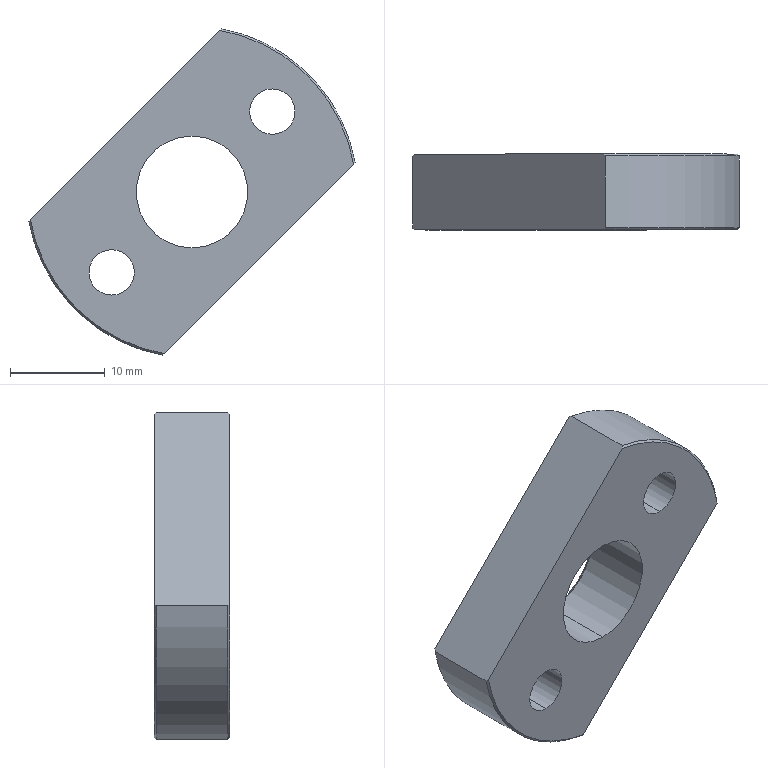Part | SolidWorks | features 3DProfileFeature 2, Chamfer 2, HoleWzd 2, ICE 2, Fillet 1, Revolution 1 | 1 solid | 24 faces | box 34.452 x 8 x 34.452 mm | volume 3811 mm3 | cylinder 12 | cone 6 | plane 6 | commonest cylinder face diameters 4.8 x4 8 x4 11.8 x2 35 x2
STEP:
#1=CARTESIAN_POINT('',(0.,23.5,-5.9));
#2=VERTEX_POINT('',#1);
#3=CARTESIAN_POINT('',(0.,23.5,5.9));
#4=VERTEX_POINT('',#3);
#5=CARTESIAN_POINT('',(0.,23.5,0.));
#6=DIRECTION('',(0.,1.,0.));
#7=DIRECTION('',(0.,0.,-1.));
#8=AXIS2_PLACEMENT_3D('',#5,#6,#7);
#9=CIRCLE('',#8,5.9);
#10=EDGE_CURVE('',#2,#4,#9,.T.);
#11=ORIENTED_EDGE('',*,*,#10,.F.);
#12=CARTESIAN_POINT('',(0.,24.,-6.4));
#13=VERTEX_POINT('',#12);
#14=CARTESIAN_POINT('',(0.,23.5,-5.9));
#15=DIRECTION('',(0.,0.7071,-0.7071));
#16=VECTOR('',#15,1000.);
#17=LINE('',#14,#16);
#18=EDGE_CURVE('',#2,#13,#17,.T.);
#19=ORIENTED_EDGE('',*,*,#18,.T.);
#20=CARTESIAN_POINT('',(0.,24.,6.4));
#21=VERTEX_POINT('',#20);
#22=CARTESIAN_POINT('',(0.,24.,0.));
#23=DIRECTION('',(0.,-1.,0.));
#24=DIRECTION('',(0.,0.,-1.));
#25=AXIS2_PLACEMENT_3D('',#22,#23,#24);
#26=CIRCLE('',#25,6.4);
#27=EDGE_CURVE('',#21,#13,#26,.T.);
#28=ORIENTED_EDGE('',*,*,#27,.F.);
#29=CARTESIAN_POINT('',(0.,23.5,5.9));
#30=DIRECTION('',(0.,0.7071,0.7071));
#31=VECTOR('',#30,1000.);
#32=LINE('',#29,#31);
#33=EDGE_CURVE('',#4,#21,#32,.T.);
#34=ORIENTED_EDGE('',*,*,#33,.F.);
#35=EDGE_LOOP('',(#11,#19,#28,#34));
#36=FACE_OUTER_BOUND('',#35,.T.);
#37=CARTESIAN_POINT('',(0.,23.5,0.));
#38=DIRECTION('',(0.,1.,0.));
#39=DIRECTION('',(0.,0.,1.));
#40=AXIS2_PLACEMENT_3D('',#37,#38,#39);
#41=CONICAL_SURFACE('',#40,5.9,0.7854);
#42=ADVANCED_FACE('',(#36),#41,.F.);
#43=CARTESIAN_POINT('',(-8.485,19.4,-12.485));
#44=VERTEX_POINT('',#43);
#45=CARTESIAN_POINT('',(-8.485,19.4,-4.485));
#46=VERTEX_POINT('',#45);
#47=CARTESIAN_POINT('',(-8.485,19.4,-8.485));
#48=DIRECTION('',(0.,1.,0.));
#49=DIRECTION('',(0.,0.,1.));
#50=AXIS2_PLACEMENT_3D('',#47,#48,#49);
#51=CIRCLE('',#50,4.);
#52=EDGE_CURVE('',#44,#46,#51,.T.);
#53=ORIENTED_EDGE('',*,*,#52,.F.);
#54=CARTESIAN_POINT('',(-8.485,24.,-12.485));
#55=VERTEX_POINT('',#54);
#56=CARTESIAN_POINT('',(-8.485,24.,-12.485));
#57=DIRECTION('',(0.,1.,0.));
#58=VECTOR('',#57,1000.);
#59=LINE('',#56,#58);
#60=EDGE_CURVE('',#44,#55,#59,.T.);
#61=ORIENTED_EDGE('',*,*,#60,.T.);
#62=CARTESIAN_POINT('',(-8.485,24.,-4.485));
#63=VERTEX_POINT('',#62);
#64=CARTESIAN_POINT('',(-8.485,24.,-8.485));
#65=DIRECTION('',(0.,1.,0.));
#66=DIRECTION('',(0.,0.,1.));
#67=AXIS2_PLACEMENT_3D('',#64,#65,#66);
#68=CIRCLE('',#67,4.);
#69=EDGE_CURVE('',#55,#63,#68,.T.);
#70=ORIENTED_EDGE('',*,*,#69,.T.);
#71=CARTESIAN_POINT('',(-8.485,24.,-4.485));
#72=DIRECTION('',(0.,1.,0.));
#73=VECTOR('',#72,1000.);
#74=LINE('',#71,#73);
#75=EDGE_CURVE('',#46,#63,#74,.T.);
#76=ORIENTED_EDGE('',*,*,#75,.F.);
#77=EDGE_LOOP('',(#53,#61,#70,#76));
#78=FACE_OUTER_BOUND('',#77,.T.);
#79=CARTESIAN_POINT('',(-8.485,24.,-8.485));
#80=DIRECTION('',(0.,1.,0.));
#81=DIRECTION('',(0.,0.,1.));
#82=AXIS2_PLACEMENT_3D('',#79,#80,#81);
#83=CYLINDRICAL_SURFACE('',#82,4.);
#84=ADVANCED_FACE('',(#78),#83,.F.);
#85=CARTESIAN_POINT('',(-8.485,16.,-10.885));
#86=VERTEX_POINT('',#85);
#87=CARTESIAN_POINT('',(-8.485,16.,-6.085));
#88=VERTEX_POINT('',#87);
#89=CARTESIAN_POINT('',(-8.485,16.,-8.485));
#90=DIRECTION('',(0.,1.,0.));
#91=DIRECTION('',(0.,0.,1.));
#92=AXIS2_PLACEMENT_3D('',#89,#90,#91);
#93=CIRCLE('',#92,2.4);
#94=EDGE_CURVE('',#86,#88,#93,.T.);
#95=ORIENTED_EDGE('',*,*,#94,.F.);
#96=CARTESIAN_POINT('',(-8.485,19.4,-10.885));
#97=VERTEX_POINT('',#96);
#98=CARTESIAN_POINT('',(-8.485,24.,-10.885));
#99=DIRECTION('',(0.,1.,0.));
#100=VECTOR('',#99,1000.);
#101=LINE('',#98,#100);
#102=EDGE_CURVE('',#86,#97,#101,.T.);
#103=ORIENTED_EDGE('',*,*,#102,.T.);
#104=CARTESIAN_POINT('',(-8.485,19.4,-6.085));
#105=VERTEX_POINT('',#104);
#106=CARTESIAN_POINT('',(-8.485,19.4,-8.485));
#107=DIRECTION('',(0.,1.,0.));
#108=DIRECTION('',(0.,0.,1.));
#109=AXIS2_PLACEMENT_3D('',#106,#107,#108);
#110=CIRCLE('',#109,2.4);
#111=EDGE_CURVE('',#97,#105,#110,.T.);
#112=ORIENTED_EDGE('',*,*,#111,.T.);
#113=CARTESIAN_POINT('',(-8.485,24.,-6.085));
#114=DIRECTION('',(0.,1.,0.));
#115=VECTOR('',#114,1000.);
#116=LINE('',#113,#115);
#117=EDGE_CURVE('',#88,#105,#116,.T.);
#118=ORIENTED_EDGE('',*,*,#117,.F.);
#119=EDGE_LOOP('',(#95,#103,#112,#118));
#120=FACE_OUTER_BOUND('',#119,.T.);
#121=CARTESIAN_POINT('',(-8.485,24.,-8.485));
#122=DIRECTION('',(0.,1.,0.));
#123=DIRECTION('',(0.,0.,1.));
#124=AXIS2_PLACEMENT_3D('',#121,#122,#123);
#125=CYLINDRICAL_SURFACE('',#124,2.4);
#126=ADVANCED_FACE('',(#120),#125,.F.);
#127=CARTESIAN_POINT('',(8.485,19.4,4.485));
#128=VERTEX_POINT('',#127);
#129=CARTESIAN_POINT('',(8.485,19.4,12.485));
#130=VERTEX_POINT('',#129);
#131=CARTESIAN_POINT('',(8.485,19.4,8.485));
#132=DIRECTION('',(0.,1.,0.));
#133=DIRECTION('',(0.,0.,1.));
#134=AXIS2_PLACEMENT_3D('',#131,#132,#133);
#135=CIRCLE('',#134,4.);
#136=EDGE_CURVE('',#128,#130,#135,.T.);
#137=ORIENTED_EDGE('',*,*,#136,.F.);
#138=CARTESIAN_POINT('',(8.485,24.,4.485));
#139=VERTEX_POINT('',#138);
#140=CARTESIAN_POINT('',(8.485,24.,4.485));
#141=DIRECTION('',(0.,1.,0.));
#142=VECTOR('',#141,1000.);
#143=LINE('',#140,#142);
#144=EDGE_CURVE('',#128,#139,#143,.T.);
#145=ORIENTED_EDGE('',*,*,#144,.T.);
#146=CARTESIAN_POINT('',(8.485,24.,12.485));
#147=VERTEX_POINT('',#146);
#148=CARTESIAN_POINT('',(8.485,24.,8.485));
#149=DIRECTION('',(0.,1.,0.));
#150=DIRECTION('',(0.,0.,1.));
#151=AXIS2_PLACEMENT_3D('',#148,#149,#150);
#152=CIRCLE('',#151,4.);
#153=EDGE_CURVE('',#139,#147,#152,.T.);
#154=ORIENTED_EDGE('',*,*,#153,.T.);
#155=CARTESIAN_POINT('',(8.485,24.,12.485));
#156=DIRECTION('',(0.,1.,0.));
#157=VECTOR('',#156,1000.);
#158=LINE('',#155,#157);
#159=EDGE_CURVE('',#130,#147,#158,.T.);
#160=ORIENTED_EDGE('',*,*,#159,.F.);
#161=EDGE_LOOP('',(#137,#145,#154,#160));
#162=FACE_OUTER_BOUND('',#161,.T.);
#163=CARTESIAN_POINT('',(8.485,24.,8.485));
#164=DIRECTION('',(0.,1.,0.));
#165=DIRECTION('',(0.,0.,1.));
#166=AXIS2_PLACEMENT_3D('',#163,#164,#165);
#167=CYLINDRICAL_SURFACE('',#166,4.);
#168=ADVANCED_FACE('',(#162),#167,.F.);
#169=CARTESIAN_POINT('',(8.485,16.,6.085));
#170=VERTEX_POINT('',#169);
#171=CARTESIAN_POINT('',(8.485,16.,10.885));
#172=VERTEX_POINT('',#171);
#173=CARTESIAN_POINT('',(8.485,16.,8.485));
#174=DIRECTION('',(0.,1.,0.));
#175=DIRECTION('',(0.,0.,1.));
#176=AXIS2_PLACEMENT_3D('',#173,#174,#175);
#177=CIRCLE('',#176,2.4);
#178=EDGE_CURVE('',#170,#172,#177,.T.);
#179=ORIENTED_EDGE('',*,*,#178,.F.);
#180=CARTESIAN_POINT('',(8.485,19.4,6.085));
#181=VERTEX_POINT('',#180);
#182=CARTESIAN_POINT('',(8.485,24.,6.085));
#183=DIRECTION('',(0.,1.,0.));
#184=VECTOR('',#183,1000.);
#185=LINE('',#182,#184);
#186=EDGE_CURVE('',#170,#181,#185,.T.);
#187=ORIENTED_EDGE('',*,*,#186,.T.);
#188=CARTESIAN_POINT('',(8.485,19.4,10.885));
#189=VERTEX_POINT('',#188);
#190=CARTESIAN_POINT('',(8.485,19.4,8.485));
#191=DIRECTION('',(0.,1.,0.));
#192=DIRECTION('',(0.,0.,1.));
#193=AXIS2_PLACEMENT_3D('',#190,#191,#192);
#194=CIRCLE('',#193,2.4);
#195=EDGE_CURVE('',#181,#189,#194,.T.);
#196=ORIENTED_EDGE('',*,*,#195,.T.);
#197=CARTESIAN_POINT('',(8.485,24.,10.885));
#198=DIRECTION('',(0.,1.,0.));
#199=VECTOR('',#198,1000.);
#200=LINE('',#197,#199);
#201=EDGE_CURVE('',#172,#189,#200,.T.);
#202=ORIENTED_EDGE('',*,*,#201,.F.);
#203=EDGE_LOOP('',(#179,#187,#196,#202));
#204=FACE_OUTER_BOUND('',#203,.T.);
#205=CARTESIAN_POINT('',(8.485,24.,8.485));
#206=DIRECTION('',(0.,1.,0.));
#207=DIRECTION('',(0.,0.,1.));
#208=AXIS2_PLACEMENT_3D('',#205,#206,#207);
#209=CYLINDRICAL_SURFACE('',#208,2.4);
#210=ADVANCED_FACE('',(#204),#209,.F.);
#211=CARTESIAN_POINT('',(0.,16.,-5.9));
#212=VERTEX_POINT('',#211);
#213=CARTESIAN_POINT('',(0.,16.,5.9));
#214=VERTEX_POINT('',#213);
#215=CARTESIAN_POINT('',(0.,16.,0.));
#216=DIRECTION('',(0.,1.,0.));
#217=DIRECTION('',(0.,0.,-1.));
#218=AXIS2_PLACEMENT_3D('',#215,#216,#217);
#219=CIRCLE('',#218,5.9);
#220=EDGE_CURVE('',#212,#214,#219,.T.);
#221=ORIENTED_EDGE('',*,*,#220,.F.);
#222=CARTESIAN_POINT('',(0.,24.,-5.9));
#223=DIRECTION('',(0.,1.,0.));
#224=VECTOR('',#223,1000.);
#225=LINE('',#222,#224);
#226=EDGE_CURVE('',#212,#2,#225,.T.);
#227=ORIENTED_EDGE('',*,*,#226,.T.);
#228=ORIENTED_EDGE('',*,*,#10,.T.);
#229=CARTESIAN_POINT('',(0.,24.,5.9));
#230=DIRECTION('',(0.,1.,0.));
#231=VECTOR('',#230,1000.);
#232=LINE('',#229,#231);
#233=EDGE_CURVE('',#214,#4,#232,.T.);
#234=ORIENTED_EDGE('',*,*,#233,.F.);
#235=EDGE_LOOP('',(#221,#227,#228,#234));
#236=FACE_OUTER_BOUND('',#235,.T.);
#237=CARTESIAN_POINT('',(0.,24.,0.));
#238=DIRECTION('',(0.,1.,0.));
#239=DIRECTION('',(0.,0.,1.));
#240=AXIS2_PLACEMENT_3D('',#237,#238,#239);
#241=CYLINDRICAL_SURFACE('',#240,5.9);
#242=ADVANCED_FACE('',(#236),#241,.F.);
#243=ORIENTED_EDGE('',*,*,#226,.F.);
#244=CARTESIAN_POINT('',(0.,16.,0.));
#245=DIRECTION('',(0.,1.,0.));
#246=DIRECTION('',(0.,0.,-1.));
#247=AXIS2_PLACEMENT_3D('',#244,#245,#246);
#248=CIRCLE('',#247,5.9);
#249=EDGE_CURVE('',#214,#212,#248,.T.);
#250=ORIENTED_EDGE('',*,*,#249,.F.);
#251=ORIENTED_EDGE('',*,*,#233,.T.);
#252=CARTESIAN_POINT('',(0.,23.5,0.));
#253=DIRECTION('',(0.,1.,0.));
#254=DIRECTION('',(0.,0.,-1.));
#255=AXIS2_PLACEMENT_3D('',#252,#253,#254);
#256=CIRCLE('',#255,5.9);
#257=EDGE_CURVE('',#4,#2,#256,.T.);
#258=ORIENTED_EDGE('',*,*,#257,.T.);
#259=EDGE_LOOP('',(#243,#250,#251,#258));
#260=FACE_OUTER_BOUND('',#259,.T.);
#261=CARTESIAN_POINT('',(0.,24.,0.));
#262=DIRECTION('',(0.,1.,0.));
#263=DIRECTION('',(0.,0.,1.));
#264=AXIS2_PLACEMENT_3D('',#261,#262,#263);
#265=CYLINDRICAL_SURFACE('',#264,5.9);
#266=ADVANCED_FACE('',(#260),#265,.F.);
#267=CARTESIAN_POINT('',(-8.485,24.,-8.485));
#268=DIRECTION('',(0.,1.,0.));
#269=DIRECTION('',(0.,0.,1.));
#270=AXIS2_PLACEMENT_3D('',#267,#268,#269);
#271=CIRCLE('',#270,4.);
#272=EDGE_CURVE('',#63,#55,#271,.T.);
#273=ORIENTED_EDGE('',*,*,#272,.F.);
#274=ORIENTED_EDGE('',*,*,#69,.F.);
#275=EDGE_LOOP('',(#273,#274));
#276=FACE_BOUND('',#275,.T.);
#277=CARTESIAN_POINT('',(8.485,24.,8.485));
#278=DIRECTION('',(0.,1.,0.));
#279=DIRECTION('',(0.,0.,1.));
#280=AXIS2_PLACEMENT_3D('',#277,#278,#279);
#281=CIRCLE('',#280,4.);
#282=EDGE_CURVE('',#147,#139,#281,.T.);
#283=ORIENTED_EDGE('',*,*,#282,.F.);
#284=ORIENTED_EDGE('',*,*,#153,.F.);
#285=EDGE_LOOP('',(#283,#284));
#286=FACE_BOUND('',#285,.T.);
#287=ORIENTED_EDGE('',*,*,#27,.T.);
#288=CARTESIAN_POINT('',(0.,24.,0.));
#289=DIRECTION('',(0.,-1.,0.));
#290=DIRECTION('',(0.,0.,-1.));
#291=AXIS2_PLACEMENT_3D('',#288,#289,#290);
#292=CIRCLE('',#291,6.4);
#293=EDGE_CURVE('',#13,#21,#292,.T.);
#294=ORIENTED_EDGE('',*,*,#293,.T.);
#295=EDGE_LOOP('',(#287,#294));
#296=FACE_BOUND('',#295,.T.);
#297=CARTESIAN_POINT('',(2.911,24.,17.053));
#298=VERTEX_POINT('',#297);
#299=CARTESIAN_POINT('',(17.053,24.,2.911));
#300=VERTEX_POINT('',#299);
#301=CARTESIAN_POINT('',(0.,24.,0.));
#302=DIRECTION('',(0.,1.,0.));
#303=DIRECTION('',(0.,0.,-1.));
#304=AXIS2_PLACEMENT_3D('',#301,#302,#303);
#305=CIRCLE('',#304,17.3);
#306=EDGE_CURVE('',#298,#300,#305,.T.);
#307=ORIENTED_EDGE('',*,*,#306,.T.);
#308=CARTESIAN_POINT('',(-2.911,24.,-17.053));
#309=VERTEX_POINT('',#308);
#310=CARTESIAN_POINT('',(7.071,24.,-7.071));
#311=DIRECTION('',(0.7071,0.,0.7071));
#312=VECTOR('',#311,1000.);
#313=LINE('',#310,#312);
#314=EDGE_CURVE('',#309,#300,#313,.T.);
#315=ORIENTED_EDGE('',*,*,#314,.F.);
#316=CARTESIAN_POINT('',(-17.053,24.,-2.911));
#317=VERTEX_POINT('',#316);
#318=CARTESIAN_POINT('',(0.,24.,0.));
#319=DIRECTION('',(0.,1.,0.));
#320=DIRECTION('',(0.,0.,-1.));
#321=AXIS2_PLACEMENT_3D('',#318,#319,#320);
#322=CIRCLE('',#321,17.3);
#323=EDGE_CURVE('',#309,#317,#322,.T.);
#324=ORIENTED_EDGE('',*,*,#323,.T.);
#325=CARTESIAN_POINT('',(-7.071,24.,7.071));
#326=DIRECTION('',(0.7071,0.,0.7071));
#327=VECTOR('',#326,1000.);
#328=LINE('',#325,#327);
#329=EDGE_CURVE('',#317,#298,#328,.T.);
#330=ORIENTED_EDGE('',*,*,#329,.T.);
#331=EDGE_LOOP('',(#307,#315,#324,#330));
#332=FACE_OUTER_BOUND('',#331,.T.);
#333=CARTESIAN_POINT('',(0.,24.,0.));
#334=DIRECTION('',(0.,-1.,0.));
#335=DIRECTION('',(0.,0.,-1.));
#336=AXIS2_PLACEMENT_3D('',#333,#334,#335);
#337=PLANE('',#336);
#338=ADVANCED_FACE('',(#276,#286,#296,#332),#337,.F.);
#339=CARTESIAN_POINT('',(-17.226,23.8,-3.084));
#340=VERTEX_POINT('',#339);
#341=CARTESIAN_POINT('',(-3.084,23.8,-17.226));
#342=VERTEX_POINT('',#341);
#343=CARTESIAN_POINT('',(0.,23.8,0.));
#344=DIRECTION('',(0.,-1.,0.));
#345=DIRECTION('',(0.,0.,-1.));
#346=AXIS2_PLACEMENT_3D('',#343,#344,#345);
#347=CIRCLE('',#346,17.5);
#348=EDGE_CURVE('',#340,#342,#347,.T.);
#349=ORIENTED_EDGE('',*,*,#348,.T.);
#350=CARTESIAN_POINT('',(-3.084,16.2,-17.226));
#351=VERTEX_POINT('',#350);
#352=CARTESIAN_POINT('',(-3.084,0.,-17.226));
#353=DIRECTION('',(0.,1.,0.));
#354=VECTOR('',#353,1000.);
#355=LINE('',#352,#354);
#356=EDGE_CURVE('',#351,#342,#355,.T.);
#357=ORIENTED_EDGE('',*,*,#356,.F.);
#358=CARTESIAN_POINT('',(-17.226,16.2,-3.084));
#359=VERTEX_POINT('',#358);
#360=CARTESIAN_POINT('',(0.,16.2,0.));
#361=DIRECTION('',(0.,1.,0.));
#362=DIRECTION('',(0.,0.,1.));
#363=AXIS2_PLACEMENT_3D('',#360,#361,#362);
#364=CIRCLE('',#363,17.5);
#365=EDGE_CURVE('',#351,#359,#364,.T.);
#366=ORIENTED_EDGE('',*,*,#365,.T.);
#367=CARTESIAN_POINT('',(-17.226,0.,-3.084));
#368=DIRECTION('',(0.,1.,0.));
#369=VECTOR('',#368,1000.);
#370=LINE('',#367,#369);
#371=EDGE_CURVE('',#359,#340,#370,.T.);
#372=ORIENTED_EDGE('',*,*,#371,.T.);
#373=EDGE_LOOP('',(#349,#357,#366,#372));
#374=FACE_OUTER_BOUND('',#373,.T.);
#375=CARTESIAN_POINT('',(0.,0.,0.));
#376=DIRECTION('',(0.,-1.,0.));
#377=DIRECTION('',(0.,0.,-1.));
#378=AXIS2_PLACEMENT_3D('',#375,#376,#377);
#379=CYLINDRICAL_SURFACE('',#378,17.5);
#380=ADVANCED_FACE('',(#374),#379,.T.);
#381=CARTESIAN_POINT('',(3.084,16.2,17.226));
#382=VERTEX_POINT('',#381);
#383=CARTESIAN_POINT('',(17.226,16.2,3.084));
#384=VERTEX_POINT('',#383);
#385=CARTESIAN_POINT('',(0.,16.2,0.));
#386=DIRECTION('',(0.,1.,0.));
#387=DIRECTION('',(0.,0.,1.));
#388=AXIS2_PLACEMENT_3D('',#385,#386,#387);
#389=CIRCLE('',#388,17.5);
#390=EDGE_CURVE('',#382,#384,#389,.T.);
#391=ORIENTED_EDGE('',*,*,#390,.T.);
#392=CARTESIAN_POINT('',(17.226,23.8,3.084));
#393=VERTEX_POINT('',#392);
#394=CARTESIAN_POINT('',(17.226,0.,3.084));
#395=DIRECTION('',(0.,1.,0.));
#396=VECTOR('',#395,1000.);
#397=LINE('',#394,#396);
#398=EDGE_CURVE('',#384,#393,#397,.T.);
#399=ORIENTED_EDGE('',*,*,#398,.T.);
#400=CARTESIAN_POINT('',(3.084,23.8,17.226));
#401=VERTEX_POINT('',#400);
#402=CARTESIAN_POINT('',(0.,23.8,0.));
#403=DIRECTION('',(0.,-1.,0.));
#404=DIRECTION('',(0.,0.,-1.));
#405=AXIS2_PLACEMENT_3D('',#402,#403,#404);
#406=CIRCLE('',#405,17.5);
#407=EDGE_CURVE('',#393,#401,#406,.T.);
#408=ORIENTED_EDGE('',*,*,#407,.T.);
#409=CARTESIAN_POINT('',(3.084,0.,17.226));
#410=DIRECTION('',(0.,1.,0.));
#411=VECTOR('',#410,1000.);
#412=LINE('',#409,#411);
#413=EDGE_CURVE('',#382,#401,#412,.T.);
#414=ORIENTED_EDGE('',*,*,#413,.F.);
#415=EDGE_LOOP('',(#391,#399,#408,#414));
#416=FACE_OUTER_BOUND('',#415,.T.);
#417=CARTESIAN_POINT('',(0.,0.,0.));
#418=DIRECTION('',(0.,-1.,0.));
#419=DIRECTION('',(0.,0.,-1.));
#420=AXIS2_PLACEMENT_3D('',#417,#418,#419);
#421=CYLINDRICAL_SURFACE('',#420,17.5);
#422=ADVANCED_FACE('',(#416),#421,.T.);
#423=CARTESIAN_POINT('',(17.053,16.,2.911));
#424=VERTEX_POINT('',#423);
#425=CARTESIAN_POINT('',(2.911,16.,17.053));
#426=VERTEX_POINT('',#425);
#427=CARTESIAN_POINT('',(0.,16.,0.));
#428=DIRECTION('',(0.,-1.,0.));
#429=DIRECTION('',(0.,0.,1.));
#430=AXIS2_PLACEMENT_3D('',#427,#428,#429);
#431=CIRCLE('',#430,17.3);
#432=EDGE_CURVE('',#424,#426,#431,.T.);
#433=ORIENTED_EDGE('',*,*,#432,.T.);
#434=CARTESIAN_POINT('',(-17.053,16.,-2.911));
#435=VERTEX_POINT('',#434);
#436=CARTESIAN_POINT('',(-15.821,16.,-1.679));
#437=DIRECTION('',(0.7071,0.,0.7071));
#438=VECTOR('',#437,1000.);
#439=LINE('',#436,#438);
#440=EDGE_CURVE('',#435,#426,#439,.T.);
#441=ORIENTED_EDGE('',*,*,#440,.F.);
#442=CARTESIAN_POINT('',(-2.911,16.,-17.053));
#443=VERTEX_POINT('',#442);
#444=CARTESIAN_POINT('',(0.,16.,0.));
#445=DIRECTION('',(0.,-1.,0.));
#446=DIRECTION('',(0.,0.,1.));
#447=AXIS2_PLACEMENT_3D('',#444,#445,#446);
#448=CIRCLE('',#447,17.3);
#449=EDGE_CURVE('',#435,#443,#448,.T.);
#450=ORIENTED_EDGE('',*,*,#449,.T.);
#451=CARTESIAN_POINT('',(-1.679,16.,-15.821));
#452=DIRECTION('',(0.7071,0.,0.7071));
#453=VECTOR('',#452,1000.);
#454=LINE('',#451,#453);
#455=EDGE_CURVE('',#443,#424,#454,.T.);
#456=ORIENTED_EDGE('',*,*,#455,.T.);
#457=EDGE_LOOP('',(#433,#441,#450,#456));
#458=FACE_OUTER_BOUND('',#457,.T.);
#459=CARTESIAN_POINT('',(8.485,16.,8.485));
#460=DIRECTION('',(0.,1.,0.));
#461=DIRECTION('',(0.,0.,1.));
#462=AXIS2_PLACEMENT_3D('',#459,#460,#461);
#463=CIRCLE('',#462,2.4);
#464=EDGE_CURVE('',#172,#170,#463,.T.);
#465=ORIENTED_EDGE('',*,*,#464,.T.);
#466=ORIENTED_EDGE('',*,*,#178,.T.);
#467=EDGE_LOOP('',(#465,#466));
#468=FACE_BOUND('',#467,.T.);
#469=CARTESIAN_POINT('',(-8.485,16.,-8.485));
#470=DIRECTION('',(0.,1.,0.));
#471=DIRECTION('',(0.,0.,1.));
#472=AXIS2_PLACEMENT_3D('',#469,#470,#471);
#473=CIRCLE('',#472,2.4);
#474=EDGE_CURVE('',#88,#86,#473,.T.);
#475=ORIENTED_EDGE('',*,*,#474,.T.);
#476=ORIENTED_EDGE('',*,*,#94,.T.);
#477=EDGE_LOOP('',(#475,#476));
#478=FACE_BOUND('',#477,.T.);
#479=ORIENTED_EDGE('',*,*,#249,.T.);
#480=ORIENTED_EDGE('',*,*,#220,.T.);
#481=EDGE_LOOP('',(#479,#480));
#482=FACE_BOUND('',#481,.T.);
#483=CARTESIAN_POINT('',(-17.5,16.,0.));
#484=DIRECTION('',(0.,1.,0.));
#485=DIRECTION('',(0.,0.,1.));
#486=AXIS2_PLACEMENT_3D('',#483,#484,#485);
#487=PLANE('',#486);
#488=ADVANCED_FACE('',(#458,#468,#478,#482),#487,.F.);
#489=CARTESIAN_POINT('',(-3.084,23.8,-17.226));
#490=CARTESIAN_POINT('',(-3.026,23.867,-17.169));
#491=CARTESIAN_POINT('',(-2.969,23.933,-17.111));
#492=CARTESIAN_POINT('',(-2.911,24.,-17.053));
#493=B_SPLINE_CURVE_WITH_KNOTS('',3,(#489,#490,#491,#492),.UNSPECIFIED.,.F.,.F.,(4,4),(0.02558,0.0259),.UNSPECIFIED.);
#494=EDGE_CURVE('',#342,#309,#493,.T.);
#495=ORIENTED_EDGE('',*,*,#494,.F.);
#496=ORIENTED_EDGE('',*,*,#348,.F.);
#497=CARTESIAN_POINT('',(-17.226,23.8,-3.084));
#498=CARTESIAN_POINT('',(-17.169,23.867,-3.026));
#499=CARTESIAN_POINT('',(-17.111,23.933,-2.969));
#500=CARTESIAN_POINT('',(-17.053,24.,-2.911));
#501=B_SPLINE_CURVE_WITH_KNOTS('',3,(#497,#498,#499,#500),.UNSPECIFIED.,.F.,.F.,(4,4),(0.02558,0.0259),.UNSPECIFIED.);
#502=EDGE_CURVE('',#340,#317,#501,.T.);
#503=ORIENTED_EDGE('',*,*,#502,.T.);
#504=ORIENTED_EDGE('',*,*,#323,.F.);
#505=EDGE_LOOP('',(#495,#496,#503,#504));
#506=FACE_OUTER_BOUND('',#505,.T.);
#507=CARTESIAN_POINT('',(0.,23.8,0.));
#508=DIRECTION('',(0.,-1.,0.));
#509=DIRECTION('',(0.,0.,-1.));
#510=AXIS2_PLACEMENT_3D('',#507,#508,#509);
#511=CONICAL_SURFACE('',#510,17.5,0.7854);
#512=ADVANCED_FACE('',(#506),#511,.T.);
#513=CARTESIAN_POINT('',(17.053,24.,2.911));
#514=CARTESIAN_POINT('',(17.111,23.933,2.969));
#515=CARTESIAN_POINT('',(17.169,23.867,3.026));
#516=CARTESIAN_POINT('',(17.226,23.8,3.084));
#517=B_SPLINE_CURVE_WITH_KNOTS('',3,(#513,#514,#515,#516),.UNSPECIFIED.,.F.,.F.,(4,4),(0.05834,0.05866),.UNSPECIFIED.);
#518=EDGE_CURVE('',#300,#393,#517,.T.);
#519=ORIENTED_EDGE('',*,*,#518,.F.);
#520=ORIENTED_EDGE('',*,*,#306,.F.);
#521=CARTESIAN_POINT('',(2.911,24.,17.053));
#522=CARTESIAN_POINT('',(2.969,23.933,17.111));
#523=CARTESIAN_POINT('',(3.026,23.867,17.169));
#524=CARTESIAN_POINT('',(3.084,23.8,17.226));
#525=B_SPLINE_CURVE_WITH_KNOTS('',3,(#521,#522,#523,#524),.UNSPECIFIED.,.F.,.F.,(4,4),(0.05834,0.05866),.UNSPECIFIED.);
#526=EDGE_CURVE('',#298,#401,#525,.T.);
#527=ORIENTED_EDGE('',*,*,#526,.T.);
#528=ORIENTED_EDGE('',*,*,#407,.F.);
#529=EDGE_LOOP('',(#519,#520,#527,#528));
#530=FACE_OUTER_BOUND('',#529,.T.);
#531=CARTESIAN_POINT('',(0.,23.8,0.));
#532=DIRECTION('',(0.,-1.,0.));
#533=DIRECTION('',(0.,0.,-1.));
#534=AXIS2_PLACEMENT_3D('',#531,#532,#533);
#535=CONICAL_SURFACE('',#534,17.5,0.7854);
#536=ADVANCED_FACE('',(#530),#535,.T.);
#537=CARTESIAN_POINT('',(17.226,16.2,3.084));
#538=CARTESIAN_POINT('',(17.169,16.133,3.026));
#539=CARTESIAN_POINT('',(17.111,16.067,2.969));
#540=CARTESIAN_POINT('',(17.053,16.,2.911));
#541=B_SPLINE_CURVE_WITH_KNOTS('',3,(#537,#538,#539,#540),.UNSPECIFIED.,.F.,.F.,(4,4),(0.02558,0.0259),.UNSPECIFIED.);
#542=EDGE_CURVE('',#384,#424,#541,.T.);
#543=ORIENTED_EDGE('',*,*,#542,.F.);
#544=ORIENTED_EDGE('',*,*,#390,.F.);
#545=CARTESIAN_POINT('',(3.084,16.2,17.226));
#546=CARTESIAN_POINT('',(3.026,16.133,17.169));
#547=CARTESIAN_POINT('',(2.969,16.067,17.111));
#548=CARTESIAN_POINT('',(2.911,16.,17.053));
#549=B_SPLINE_CURVE_WITH_KNOTS('',3,(#545,#546,#547,#548),.UNSPECIFIED.,.F.,.F.,(4,4),(0.02558,0.0259),.UNSPECIFIED.);
#550=EDGE_CURVE('',#382,#426,#549,.T.);
#551=ORIENTED_EDGE('',*,*,#550,.T.);
#552=ORIENTED_EDGE('',*,*,#432,.F.);
#553=EDGE_LOOP('',(#543,#544,#551,#552));
#554=FACE_OUTER_BOUND('',#553,.T.);
#555=CARTESIAN_POINT('',(0.,16.,0.));
#556=DIRECTION('',(0.,1.,0.));
#557=DIRECTION('',(0.,0.,1.));
#558=AXIS2_PLACEMENT_3D('',#555,#556,#557);
#559=CONICAL_SURFACE('',#558,17.3,0.7854);
#560=ADVANCED_FACE('',(#554),#559,.T.);
#561=CARTESIAN_POINT('',(-2.911,16.,-17.053));
#562=CARTESIAN_POINT('',(-2.969,16.067,-17.111));
#563=CARTESIAN_POINT('',(-3.026,16.133,-17.169));
#564=CARTESIAN_POINT('',(-3.084,16.2,-17.226));
#565=B_SPLINE_CURVE_WITH_KNOTS('',3,(#561,#562,#563,#564),.UNSPECIFIED.,.F.,.F.,(4,4),(0.05834,0.05866),.UNSPECIFIED.);
#566=EDGE_CURVE('',#443,#351,#565,.T.);
#567=ORIENTED_EDGE('',*,*,#566,.F.);
#568=ORIENTED_EDGE('',*,*,#449,.F.);
#569=CARTESIAN_POINT('',(-17.053,16.,-2.911));
#570=CARTESIAN_POINT('',(-17.111,16.067,-2.969));
#571=CARTESIAN_POINT('',(-17.169,16.133,-3.026));
#572=CARTESIAN_POINT('',(-17.226,16.2,-3.084));
#573=B_SPLINE_CURVE_WITH_KNOTS('',3,(#569,#570,#571,#572),.UNSPECIFIED.,.F.,.F.,(4,4),(0.05834,0.05866),.UNSPECIFIED.);
#574=EDGE_CURVE('',#435,#359,#573,.T.);
#575=ORIENTED_EDGE('',*,*,#574,.T.);
#576=ORIENTED_EDGE('',*,*,#365,.F.);
#577=EDGE_LOOP('',(#567,#568,#575,#576));
#578=FACE_OUTER_BOUND('',#577,.T.);
#579=CARTESIAN_POINT('',(0.,16.,0.));
#580=DIRECTION('',(0.,1.,0.));
#581=DIRECTION('',(0.,0.,1.));
#582=AXIS2_PLACEMENT_3D('',#579,#580,#581);
#583=CONICAL_SURFACE('',#582,17.3,0.7854);
#584=ADVANCED_FACE('',(#578),#583,.T.);
#585=ORIENTED_EDGE('',*,*,#186,.F.);
#586=ORIENTED_EDGE('',*,*,#464,.F.);
#587=ORIENTED_EDGE('',*,*,#201,.T.);
#588=CARTESIAN_POINT('',(8.485,19.4,8.485));
#589=DIRECTION('',(0.,1.,0.));
#590=DIRECTION('',(0.,0.,1.));
#591=AXIS2_PLACEMENT_3D('',#588,#589,#590);
#592=CIRCLE('',#591,2.4);
#593=EDGE_CURVE('',#189,#181,#592,.T.);
#594=ORIENTED_EDGE('',*,*,#593,.T.);
#595=EDGE_LOOP('',(#585,#586,#587,#594));
#596=FACE_OUTER_BOUND('',#595,.T.);
#597=CARTESIAN_POINT('',(8.485,24.,8.485));
#598=DIRECTION('',(0.,1.,0.));
#599=DIRECTION('',(0.,0.,1.));
#600=AXIS2_PLACEMENT_3D('',#597,#598,#599);
#601=CYLINDRICAL_SURFACE('',#600,2.4);
#602=ADVANCED_FACE('',(#596),#601,.F.);
#603=ORIENTED_EDGE('',*,*,#593,.F.);
#604=ORIENTED_EDGE('',*,*,#195,.F.);
#605=EDGE_LOOP('',(#603,#604));
#606=FACE_BOUND('',#605,.T.);
#607=CARTESIAN_POINT('',(8.485,19.4,8.485));
#608=DIRECTION('',(0.,1.,0.));
#609=DIRECTION('',(0.,0.,1.));
#610=AXIS2_PLACEMENT_3D('',#607,#608,#609);
#611=CIRCLE('',#610,4.);
#612=EDGE_CURVE('',#130,#128,#611,.T.);
#613=ORIENTED_EDGE('',*,*,#612,.T.);
#614=ORIENTED_EDGE('',*,*,#136,.T.);
#615=EDGE_LOOP('',(#613,#614));
#616=FACE_OUTER_BOUND('',#615,.T.);
#617=CARTESIAN_POINT('',(10.885,19.4,8.485));
#618=DIRECTION('',(0.,-1.,0.));
#619=DIRECTION('',(0.,0.,-1.));
#620=AXIS2_PLACEMENT_3D('',#617,#618,#619);
#621=PLANE('',#620);
#622=ADVANCED_FACE('',(#606,#616),#621,.F.);
#623=ORIENTED_EDGE('',*,*,#144,.F.);
#624=ORIENTED_EDGE('',*,*,#612,.F.);
#625=ORIENTED_EDGE('',*,*,#159,.T.);
#626=ORIENTED_EDGE('',*,*,#282,.T.);
#627=EDGE_LOOP('',(#623,#624,#625,#626));
#628=FACE_OUTER_BOUND('',#627,.T.);
#629=CARTESIAN_POINT('',(8.485,24.,8.485));
#630=DIRECTION('',(0.,1.,0.));
#631=DIRECTION('',(0.,0.,1.));
#632=AXIS2_PLACEMENT_3D('',#629,#630,#631);
#633=CYLINDRICAL_SURFACE('',#632,4.);
#634=ADVANCED_FACE('',(#628),#633,.F.);
#635=ORIENTED_EDGE('',*,*,#102,.F.);
#636=ORIENTED_EDGE('',*,*,#474,.F.);
#637=ORIENTED_EDGE('',*,*,#117,.T.);
#638=CARTESIAN_POINT('',(-8.485,19.4,-8.485));
#639=DIRECTION('',(0.,1.,0.));
#640=DIRECTION('',(0.,0.,1.));
#641=AXIS2_PLACEMENT_3D('',#638,#639,#640);
#642=CIRCLE('',#641,2.4);
#643=EDGE_CURVE('',#105,#97,#642,.T.);
#644=ORIENTED_EDGE('',*,*,#643,.T.);
#645=EDGE_LOOP('',(#635,#636,#637,#644));
#646=FACE_OUTER_BOUND('',#645,.T.);
#647=CARTESIAN_POINT('',(-8.485,24.,-8.485));
#648=DIRECTION('',(0.,1.,0.));
#649=DIRECTION('',(0.,0.,1.));
#650=AXIS2_PLACEMENT_3D('',#647,#648,#649);
#651=CYLINDRICAL_SURFACE('',#650,2.4);
#652=ADVANCED_FACE('',(#646),#651,.F.);
#653=ORIENTED_EDGE('',*,*,#643,.F.);
#654=ORIENTED_EDGE('',*,*,#111,.F.);
#655=EDGE_LOOP('',(#653,#654));
#656=FACE_BOUND('',#655,.T.);
#657=CARTESIAN_POINT('',(-8.485,19.4,-8.485));
#658=DIRECTION('',(0.,1.,0.));
#659=DIRECTION('',(0.,0.,1.));
#660=AXIS2_PLACEMENT_3D('',#657,#658,#659);
#661=CIRCLE('',#660,4.);
#662=EDGE_CURVE('',#46,#44,#661,.T.);
#663=ORIENTED_EDGE('',*,*,#662,.T.);
#664=ORIENTED_EDGE('',*,*,#52,.T.);
#665=EDGE_LOOP('',(#663,#664));
#666=FACE_OUTER_BOUND('',#665,.T.);
#667=CARTESIAN_POINT('',(-6.085,19.4,-8.485));
#668=DIRECTION('',(0.,-1.,0.));
#669=DIRECTION('',(0.,0.,-1.));
#670=AXIS2_PLACEMENT_3D('',#667,#668,#669);
#671=PLANE('',#670);
#672=ADVANCED_FACE('',(#656,#666),#671,.F.);
#673=ORIENTED_EDGE('',*,*,#60,.F.);
#674=ORIENTED_EDGE('',*,*,#662,.F.);
#675=ORIENTED_EDGE('',*,*,#75,.T.);
#676=ORIENTED_EDGE('',*,*,#272,.T.);
#677=EDGE_LOOP('',(#673,#674,#675,#676));
#678=FACE_OUTER_BOUND('',#677,.T.);
#679=CARTESIAN_POINT('',(-8.485,24.,-8.485));
#680=DIRECTION('',(0.,1.,0.));
#681=DIRECTION('',(0.,0.,1.));
#682=AXIS2_PLACEMENT_3D('',#679,#680,#681);
#683=CYLINDRICAL_SURFACE('',#682,4.);
#684=ADVANCED_FACE('',(#678),#683,.F.);
#685=ORIENTED_EDGE('',*,*,#18,.F.);
#686=ORIENTED_EDGE('',*,*,#257,.F.);
#687=ORIENTED_EDGE('',*,*,#33,.T.);
#688=ORIENTED_EDGE('',*,*,#293,.F.);
#689=EDGE_LOOP('',(#685,#686,#687,#688));
#690=FACE_OUTER_BOUND('',#689,.T.);
#691=CARTESIAN_POINT('',(0.,23.5,0.));
#692=DIRECTION('',(0.,1.,0.));
#693=DIRECTION('',(0.,0.,1.));
#694=AXIS2_PLACEMENT_3D('',#691,#692,#693);
#695=CONICAL_SURFACE('',#694,5.9,0.7854);
#696=ADVANCED_FACE('',(#690),#695,.F.);
#697=ORIENTED_EDGE('',*,*,#371,.F.);
#698=ORIENTED_EDGE('',*,*,#574,.F.);
#699=ORIENTED_EDGE('',*,*,#440,.T.);
#700=ORIENTED_EDGE('',*,*,#550,.F.);
#701=ORIENTED_EDGE('',*,*,#413,.T.);
#702=ORIENTED_EDGE('',*,*,#526,.F.);
#703=ORIENTED_EDGE('',*,*,#329,.F.);
#704=ORIENTED_EDGE('',*,*,#502,.F.);
#705=EDGE_LOOP('',(#697,#698,#699,#700,#701,#702,#703,#704));
#706=FACE_OUTER_BOUND('',#705,.T.);
#707=CARTESIAN_POINT('',(-7.071,0.,7.071));
#708=DIRECTION('',(-0.7071,0.,0.7071));
#709=DIRECTION('',(0.7071,0.,0.7071));
#710=AXIS2_PLACEMENT_3D('',#707,#708,#709);
#711=PLANE('',#710);
#712=ADVANCED_FACE('',(#706),#711,.T.);
#713=ORIENTED_EDGE('',*,*,#494,.T.);
#714=ORIENTED_EDGE('',*,*,#314,.T.);
#715=ORIENTED_EDGE('',*,*,#518,.T.);
#716=ORIENTED_EDGE('',*,*,#398,.F.);
#717=ORIENTED_EDGE('',*,*,#542,.T.);
#718=ORIENTED_EDGE('',*,*,#455,.F.);
#719=ORIENTED_EDGE('',*,*,#566,.T.);
#720=ORIENTED_EDGE('',*,*,#356,.T.);
#721=EDGE_LOOP('',(#713,#714,#715,#716,#717,#718,#719,#720));
#722=FACE_OUTER_BOUND('',#721,.T.);
#723=CARTESIAN_POINT('',(7.071,0.,-7.071));
#724=DIRECTION('',(-0.7071,0.,0.7071));
#725=DIRECTION('',(0.7071,0.,0.7071));
#726=AXIS2_PLACEMENT_3D('',#723,#724,#725);
#727=PLANE('',#726);
#728=ADVANCED_FACE('',(#722),#727,.F.);
#729=CLOSED_SHELL('',(#42,#84,#126,#168,#210,#242,#266,#338,#380,#422,#488,#512,#536,#560,#584,#602,#622,#634,#652,#672,#684,#696,#712,#728));
#730=MANIFOLD_SOLID_BREP('',#729);
#731=CARTESIAN_POINT('',(0.,0.,0.));
#732=DIRECTION('',(0.,0.,1.));
#733=DIRECTION('',(1.,0.,0.));
#734=AXIS2_PLACEMENT_3D('',#731,#732,#733);
#735=(LENGTH_UNIT()NAMED_UNIT(*)SI_UNIT(.MILLI.,.METRE.));
#736=UNCERTAINTY_MEASURE_WITH_UNIT(LENGTH_MEASURE(0.00001),#735,'','');
#737=(NAMED_UNIT(*)PLANE_ANGLE_UNIT()SI_UNIT($,.RADIAN.));
#738=(NAMED_UNIT(*)SI_UNIT($,.STERADIAN.)SOLID_ANGLE_UNIT());
#739=(GEOMETRIC_REPRESENTATION_CONTEXT(3)GLOBAL_UNCERTAINTY_ASSIGNED_CONTEXT((#736))GLOBAL_UNIT_ASSIGNED_CONTEXT((#735,#737,#738))REPRESENTATION_CONTEXT('',''));
#740=ADVANCED_BREP_SHAPE_REPRESENTATION('',(#730,#734),#739);